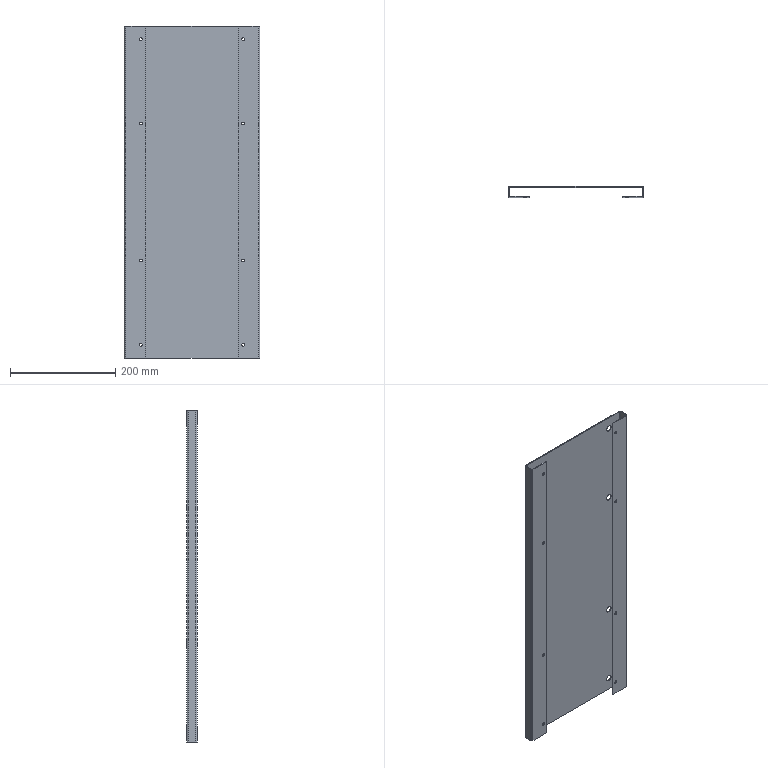Part | STEP file | ASND-0110-E63-HLTP01-006 | 1 solid | 54 faces | box 257 x 20 x 630 mm | volume 345415 mm3 | cylinder 40 | plane 14 | commonest cylinder face diameters 5.495 x16 11.495 x16 3 x4 6 x4